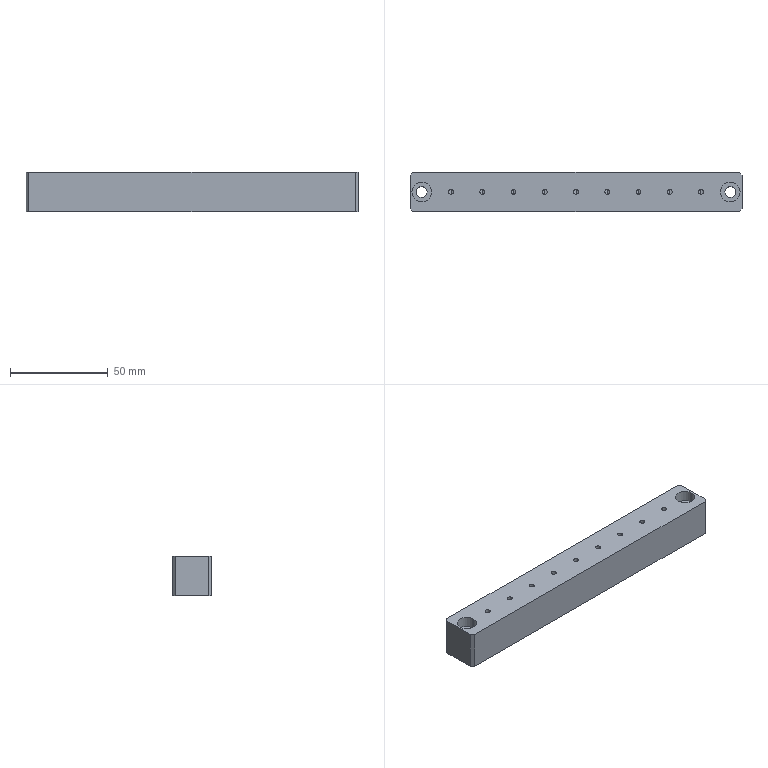Part | STEP file | PN_0013 | 1 solid | 74 faces | box 170 x 20 x 20 mm | volume 64184 mm3 | cylinder 44 | cone 18 | plane 12 | commonest cylinder face diameters 2.5 x18 4.2 x18 5.5 x4 10 x4